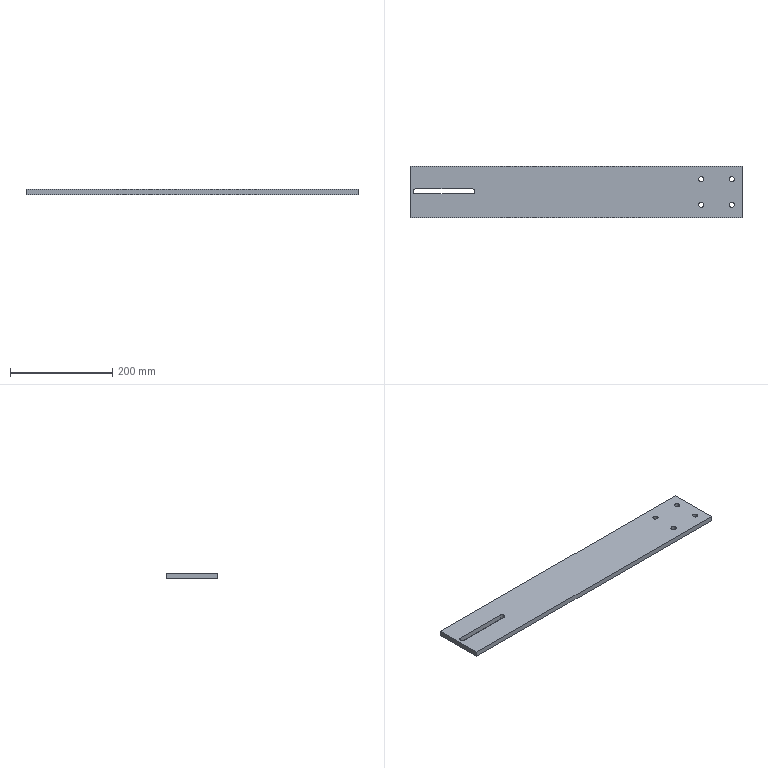Part | SolidWorks | features ICE 2, Extrusion 1 | 1 solid | 22 faces | box 650 x 100 x 10 mm | volume 635032 mm3 | cylinder 12 | plane 10 | commonest cylinder face diameters 10 x8 9 x4
STEP:
#1=CARTESIAN_POINT('',(300.,-25.,0.));
#2=VERTEX_POINT('',#1);
#3=CARTESIAN_POINT('',(310.,-25.,0.));
#4=VERTEX_POINT('',#3);
#5=CARTESIAN_POINT('',(305.,-25.,0.));
#6=DIRECTION('',(0.,0.,1.));
#7=DIRECTION('',(1.,0.,0.));
#8=AXIS2_PLACEMENT_3D('',#5,#6,#7);
#9=CIRCLE('',#8,5.);
#10=EDGE_CURVE('',#2,#4,#9,.T.);
#11=ORIENTED_EDGE('',*,*,#10,.F.);
#12=CARTESIAN_POINT('',(300.,-25.,10.));
#13=VERTEX_POINT('',#12);
#14=CARTESIAN_POINT('',(300.,-25.,0.));
#15=DIRECTION('',(0.,0.,1.));
#16=VECTOR('',#15,1000.);
#17=LINE('',#14,#16);
#18=EDGE_CURVE('',#2,#13,#17,.T.);
#19=ORIENTED_EDGE('',*,*,#18,.T.);
#20=CARTESIAN_POINT('',(310.,-25.,10.));
#21=VERTEX_POINT('',#20);
#22=CARTESIAN_POINT('',(305.,-25.,10.));
#23=DIRECTION('',(0.,0.,1.));
#24=DIRECTION('',(1.,0.,0.));
#25=AXIS2_PLACEMENT_3D('',#22,#23,#24);
#26=CIRCLE('',#25,5.);
#27=EDGE_CURVE('',#13,#21,#26,.T.);
#28=ORIENTED_EDGE('',*,*,#27,.T.);
#29=CARTESIAN_POINT('',(310.,-25.,0.));
#30=DIRECTION('',(0.,0.,1.));
#31=VECTOR('',#30,1000.);
#32=LINE('',#29,#31);
#33=EDGE_CURVE('',#4,#21,#32,.T.);
#34=ORIENTED_EDGE('',*,*,#33,.F.);
#35=EDGE_LOOP('',(#11,#19,#28,#34));
#36=FACE_OUTER_BOUND('',#35,.T.);
#37=CARTESIAN_POINT('',(305.,-25.,0.));
#38=DIRECTION('',(0.,0.,1.));
#39=DIRECTION('',(1.,0.,0.));
#40=AXIS2_PLACEMENT_3D('',#37,#38,#39);
#41=CYLINDRICAL_SURFACE('',#40,5.);
#42=ADVANCED_FACE('',(#36),#41,.F.);
#43=CARTESIAN_POINT('',(240.,-25.,0.));
#44=VERTEX_POINT('',#43);
#45=CARTESIAN_POINT('',(250.,-25.,0.));
#46=VERTEX_POINT('',#45);
#47=CARTESIAN_POINT('',(245.,-25.,0.));
#48=DIRECTION('',(0.,0.,1.));
#49=DIRECTION('',(1.,0.,0.));
#50=AXIS2_PLACEMENT_3D('',#47,#48,#49);
#51=CIRCLE('',#50,5.);
#52=EDGE_CURVE('',#44,#46,#51,.T.);
#53=ORIENTED_EDGE('',*,*,#52,.F.);
#54=CARTESIAN_POINT('',(240.,-25.,10.));
#55=VERTEX_POINT('',#54);
#56=CARTESIAN_POINT('',(240.,-25.,0.));
#57=DIRECTION('',(0.,0.,1.));
#58=VECTOR('',#57,1000.);
#59=LINE('',#56,#58);
#60=EDGE_CURVE('',#44,#55,#59,.T.);
#61=ORIENTED_EDGE('',*,*,#60,.T.);
#62=CARTESIAN_POINT('',(250.,-25.,10.));
#63=VERTEX_POINT('',#62);
#64=CARTESIAN_POINT('',(245.,-25.,10.));
#65=DIRECTION('',(0.,0.,1.));
#66=DIRECTION('',(1.,0.,0.));
#67=AXIS2_PLACEMENT_3D('',#64,#65,#66);
#68=CIRCLE('',#67,5.);
#69=EDGE_CURVE('',#55,#63,#68,.T.);
#70=ORIENTED_EDGE('',*,*,#69,.T.);
#71=CARTESIAN_POINT('',(250.,-25.,0.));
#72=DIRECTION('',(0.,0.,1.));
#73=VECTOR('',#72,1000.);
#74=LINE('',#71,#73);
#75=EDGE_CURVE('',#46,#63,#74,.T.);
#76=ORIENTED_EDGE('',*,*,#75,.F.);
#77=EDGE_LOOP('',(#53,#61,#70,#76));
#78=FACE_OUTER_BOUND('',#77,.T.);
#79=CARTESIAN_POINT('',(245.,-25.,0.));
#80=DIRECTION('',(0.,0.,1.));
#81=DIRECTION('',(1.,0.,0.));
#82=AXIS2_PLACEMENT_3D('',#79,#80,#81);
#83=CYLINDRICAL_SURFACE('',#82,5.);
#84=ADVANCED_FACE('',(#78),#83,.F.);
#85=CARTESIAN_POINT('',(240.,25.,0.));
#86=VERTEX_POINT('',#85);
#87=CARTESIAN_POINT('',(250.,25.,0.));
#88=VERTEX_POINT('',#87);
#89=CARTESIAN_POINT('',(245.,25.,0.));
#90=DIRECTION('',(0.,0.,1.));
#91=DIRECTION('',(1.,0.,0.));
#92=AXIS2_PLACEMENT_3D('',#89,#90,#91);
#93=CIRCLE('',#92,5.);
#94=EDGE_CURVE('',#86,#88,#93,.T.);
#95=ORIENTED_EDGE('',*,*,#94,.F.);
#96=CARTESIAN_POINT('',(240.,25.,10.));
#97=VERTEX_POINT('',#96);
#98=CARTESIAN_POINT('',(240.,25.,0.));
#99=DIRECTION('',(0.,0.,1.));
#100=VECTOR('',#99,1000.);
#101=LINE('',#98,#100);
#102=EDGE_CURVE('',#86,#97,#101,.T.);
#103=ORIENTED_EDGE('',*,*,#102,.T.);
#104=CARTESIAN_POINT('',(250.,25.,10.));
#105=VERTEX_POINT('',#104);
#106=CARTESIAN_POINT('',(245.,25.,10.));
#107=DIRECTION('',(0.,0.,1.));
#108=DIRECTION('',(1.,0.,0.));
#109=AXIS2_PLACEMENT_3D('',#106,#107,#108);
#110=CIRCLE('',#109,5.);
#111=EDGE_CURVE('',#97,#105,#110,.T.);
#112=ORIENTED_EDGE('',*,*,#111,.T.);
#113=CARTESIAN_POINT('',(250.,25.,0.));
#114=DIRECTION('',(0.,0.,1.));
#115=VECTOR('',#114,1000.);
#116=LINE('',#113,#115);
#117=EDGE_CURVE('',#88,#105,#116,.T.);
#118=ORIENTED_EDGE('',*,*,#117,.F.);
#119=EDGE_LOOP('',(#95,#103,#112,#118));
#120=FACE_OUTER_BOUND('',#119,.T.);
#121=CARTESIAN_POINT('',(245.,25.,0.));
#122=DIRECTION('',(0.,0.,1.));
#123=DIRECTION('',(1.,0.,0.));
#124=AXIS2_PLACEMENT_3D('',#121,#122,#123);
#125=CYLINDRICAL_SURFACE('',#124,5.);
#126=ADVANCED_FACE('',(#120),#125,.F.);
#127=CARTESIAN_POINT('',(300.,25.,0.));
#128=VERTEX_POINT('',#127);
#129=CARTESIAN_POINT('',(310.,25.,0.));
#130=VERTEX_POINT('',#129);
#131=CARTESIAN_POINT('',(305.,25.,0.));
#132=DIRECTION('',(0.,0.,1.));
#133=DIRECTION('',(1.,0.,0.));
#134=AXIS2_PLACEMENT_3D('',#131,#132,#133);
#135=CIRCLE('',#134,5.);
#136=EDGE_CURVE('',#128,#130,#135,.T.);
#137=ORIENTED_EDGE('',*,*,#136,.F.);
#138=CARTESIAN_POINT('',(300.,25.,10.));
#139=VERTEX_POINT('',#138);
#140=CARTESIAN_POINT('',(300.,25.,0.));
#141=DIRECTION('',(0.,0.,1.));
#142=VECTOR('',#141,1000.);
#143=LINE('',#140,#142);
#144=EDGE_CURVE('',#128,#139,#143,.T.);
#145=ORIENTED_EDGE('',*,*,#144,.T.);
#146=CARTESIAN_POINT('',(310.,25.,10.));
#147=VERTEX_POINT('',#146);
#148=CARTESIAN_POINT('',(305.,25.,10.));
#149=DIRECTION('',(0.,0.,1.));
#150=DIRECTION('',(1.,0.,0.));
#151=AXIS2_PLACEMENT_3D('',#148,#149,#150);
#152=CIRCLE('',#151,5.);
#153=EDGE_CURVE('',#139,#147,#152,.T.);
#154=ORIENTED_EDGE('',*,*,#153,.T.);
#155=CARTESIAN_POINT('',(310.,25.,0.));
#156=DIRECTION('',(0.,0.,1.));
#157=VECTOR('',#156,1000.);
#158=LINE('',#155,#157);
#159=EDGE_CURVE('',#130,#147,#158,.T.);
#160=ORIENTED_EDGE('',*,*,#159,.F.);
#161=EDGE_LOOP('',(#137,#145,#154,#160));
#162=FACE_OUTER_BOUND('',#161,.T.);
#163=CARTESIAN_POINT('',(305.,25.,0.));
#164=DIRECTION('',(0.,0.,1.));
#165=DIRECTION('',(1.,0.,0.));
#166=AXIS2_PLACEMENT_3D('',#163,#164,#165);
#167=CYLINDRICAL_SURFACE('',#166,5.);
#168=ADVANCED_FACE('',(#162),#167,.F.);
#169=CARTESIAN_POINT('',(-325.,50.,0.));
#170=VERTEX_POINT('',#169);
#171=CARTESIAN_POINT('',(-325.,-50.,0.));
#172=VERTEX_POINT('',#171);
#173=CARTESIAN_POINT('',(-325.,-50.,0.));
#174=DIRECTION('',(0.,-1.,0.));
#175=VECTOR('',#174,1000.);
#176=LINE('',#173,#175);
#177=EDGE_CURVE('',#170,#172,#176,.T.);
#178=ORIENTED_EDGE('',*,*,#177,.T.);
#179=CARTESIAN_POINT('',(-325.,-50.,10.));
#180=VERTEX_POINT('',#179);
#181=CARTESIAN_POINT('',(-325.,-50.,10.));
#182=DIRECTION('',(0.,0.,-1.));
#183=VECTOR('',#182,1000.);
#184=LINE('',#181,#183);
#185=EDGE_CURVE('',#180,#172,#184,.T.);
#186=ORIENTED_EDGE('',*,*,#185,.F.);
#187=CARTESIAN_POINT('',(-325.,50.,10.));
#188=VERTEX_POINT('',#187);
#189=CARTESIAN_POINT('',(-325.,-50.,10.));
#190=DIRECTION('',(0.,-1.,0.));
#191=VECTOR('',#190,1000.);
#192=LINE('',#189,#191);
#193=EDGE_CURVE('',#188,#180,#192,.T.);
#194=ORIENTED_EDGE('',*,*,#193,.F.);
#195=CARTESIAN_POINT('',(-325.,50.,10.));
#196=DIRECTION('',(0.,0.,-1.));
#197=VECTOR('',#196,1000.);
#198=LINE('',#195,#197);
#199=EDGE_CURVE('',#188,#170,#198,.T.);
#200=ORIENTED_EDGE('',*,*,#199,.T.);
#201=EDGE_LOOP('',(#178,#186,#194,#200));
#202=FACE_OUTER_BOUND('',#201,.T.);
#203=CARTESIAN_POINT('',(-325.,-50.,10.));
#204=DIRECTION('',(1.,0.,0.));
#205=DIRECTION('',(0.,0.,-1.));
#206=AXIS2_PLACEMENT_3D('',#203,#204,#205);
#207=PLANE('',#206);
#208=ADVANCED_FACE('',(#202),#207,.F.);
#209=CARTESIAN_POINT('',(325.,-50.,0.));
#210=VERTEX_POINT('',#209);
#211=CARTESIAN_POINT('',(325.,-50.,0.));
#212=DIRECTION('',(1.,0.,0.));
#213=VECTOR('',#212,1000.);
#214=LINE('',#211,#213);
#215=EDGE_CURVE('',#172,#210,#214,.T.);
#216=ORIENTED_EDGE('',*,*,#215,.T.);
#217=CARTESIAN_POINT('',(325.,-50.,10.));
#218=VERTEX_POINT('',#217);
#219=CARTESIAN_POINT('',(325.,-50.,10.));
#220=DIRECTION('',(0.,0.,-1.));
#221=VECTOR('',#220,1000.);
#222=LINE('',#219,#221);
#223=EDGE_CURVE('',#218,#210,#222,.T.);
#224=ORIENTED_EDGE('',*,*,#223,.F.);
#225=CARTESIAN_POINT('',(325.,-50.,10.));
#226=DIRECTION('',(1.,0.,0.));
#227=VECTOR('',#226,1000.);
#228=LINE('',#225,#227);
#229=EDGE_CURVE('',#180,#218,#228,.T.);
#230=ORIENTED_EDGE('',*,*,#229,.F.);
#231=ORIENTED_EDGE('',*,*,#185,.T.);
#232=EDGE_LOOP('',(#216,#224,#230,#231));
#233=FACE_OUTER_BOUND('',#232,.T.);
#234=CARTESIAN_POINT('',(325.,-50.,10.));
#235=DIRECTION('',(0.,1.,0.));
#236=DIRECTION('',(-1.,0.,0.));
#237=AXIS2_PLACEMENT_3D('',#234,#235,#236);
#238=PLANE('',#237);
#239=ADVANCED_FACE('',(#233),#238,.F.);
#240=CARTESIAN_POINT('',(325.,50.,0.));
#241=VERTEX_POINT('',#240);
#242=CARTESIAN_POINT('',(325.,-50.,0.));
#243=DIRECTION('',(0.,1.,0.));
#244=VECTOR('',#243,1000.);
#245=LINE('',#242,#244);
#246=EDGE_CURVE('',#210,#241,#245,.T.);
#247=ORIENTED_EDGE('',*,*,#246,.T.);
#248=CARTESIAN_POINT('',(325.,50.,10.));
#249=VERTEX_POINT('',#248);
#250=CARTESIAN_POINT('',(325.,50.,10.));
#251=DIRECTION('',(0.,0.,-1.));
#252=VECTOR('',#251,1000.);
#253=LINE('',#250,#252);
#254=EDGE_CURVE('',#249,#241,#253,.T.);
#255=ORIENTED_EDGE('',*,*,#254,.F.);
#256=CARTESIAN_POINT('',(325.,-50.,10.));
#257=DIRECTION('',(0.,1.,0.));
#258=VECTOR('',#257,1000.);
#259=LINE('',#256,#258);
#260=EDGE_CURVE('',#218,#249,#259,.T.);
#261=ORIENTED_EDGE('',*,*,#260,.F.);
#262=ORIENTED_EDGE('',*,*,#223,.T.);
#263=EDGE_LOOP('',(#247,#255,#261,#262));
#264=FACE_OUTER_BOUND('',#263,.T.);
#265=CARTESIAN_POINT('',(325.,-50.,10.));
#266=DIRECTION('',(-1.,0.,0.));
#267=DIRECTION('',(0.,0.,1.));
#268=AXIS2_PLACEMENT_3D('',#265,#266,#267);
#269=PLANE('',#268);
#270=ADVANCED_FACE('',(#264),#269,.F.);
#271=CARTESIAN_POINT('',(325.,50.,0.));
#272=DIRECTION('',(-1.,0.,0.));
#273=VECTOR('',#272,1000.);
#274=LINE('',#271,#273);
#275=EDGE_CURVE('',#241,#170,#274,.T.);
#276=ORIENTED_EDGE('',*,*,#275,.T.);
#277=ORIENTED_EDGE('',*,*,#199,.F.);
#278=CARTESIAN_POINT('',(325.,50.,10.));
#279=DIRECTION('',(-1.,0.,0.));
#280=VECTOR('',#279,1000.);
#281=LINE('',#278,#280);
#282=EDGE_CURVE('',#249,#188,#281,.T.);
#283=ORIENTED_EDGE('',*,*,#282,.F.);
#284=ORIENTED_EDGE('',*,*,#254,.T.);
#285=EDGE_LOOP('',(#276,#277,#283,#284));
#286=FACE_OUTER_BOUND('',#285,.T.);
#287=CARTESIAN_POINT('',(325.,50.,10.));
#288=DIRECTION('',(0.,-1.,0.));
#289=DIRECTION('',(1.,0.,0.));
#290=AXIS2_PLACEMENT_3D('',#287,#288,#289);
#291=PLANE('',#290);
#292=ADVANCED_FACE('',(#286),#291,.F.);
#293=CARTESIAN_POINT('',(-202.885,-3.814,10.));
#294=VERTEX_POINT('',#293);
#295=CARTESIAN_POINT('',(-198.385,0.6857,10.));
#296=VERTEX_POINT('',#295);
#297=CARTESIAN_POINT('',(-202.885,0.6857,10.));
#298=DIRECTION('',(0.,0.,1.));
#299=DIRECTION('',(1.,0.,0.));
#300=AXIS2_PLACEMENT_3D('',#297,#298,#299);
#301=CIRCLE('',#300,4.5);
#302=EDGE_CURVE('',#294,#296,#301,.T.);
#303=ORIENTED_EDGE('',*,*,#302,.F.);
#304=CARTESIAN_POINT('',(-313.885,-3.814,10.));
#305=VERTEX_POINT('',#304);
#306=CARTESIAN_POINT('',(-313.885,-3.814,10.));
#307=DIRECTION('',(1.,0.,0.));
#308=VECTOR('',#307,1000.);
#309=LINE('',#306,#308);
#310=EDGE_CURVE('',#305,#294,#309,.T.);
#311=ORIENTED_EDGE('',*,*,#310,.F.);
#312=CARTESIAN_POINT('',(-318.385,0.6857,10.));
#313=VERTEX_POINT('',#312);
#314=CARTESIAN_POINT('',(-313.885,0.6857,10.));
#315=DIRECTION('',(0.,0.,1.));
#316=DIRECTION('',(-1.,0.,0.));
#317=AXIS2_PLACEMENT_3D('',#314,#315,#316);
#318=CIRCLE('',#317,4.5);
#319=EDGE_CURVE('',#313,#305,#318,.T.);
#320=ORIENTED_EDGE('',*,*,#319,.F.);
#321=CARTESIAN_POINT('',(-318.385,1.686,10.));
#322=VERTEX_POINT('',#321);
#323=CARTESIAN_POINT('',(-318.385,0.6857,10.));
#324=DIRECTION('',(0.,-1.,0.));
#325=VECTOR('',#324,1000.);
#326=LINE('',#323,#325);
#327=EDGE_CURVE('',#322,#313,#326,.T.);
#328=ORIENTED_EDGE('',*,*,#327,.F.);
#329=CARTESIAN_POINT('',(-313.885,6.186,10.));
#330=VERTEX_POINT('',#329);
#331=CARTESIAN_POINT('',(-313.885,1.686,10.));
#332=DIRECTION('',(0.,0.,1.));
#333=DIRECTION('',(-1.,0.,0.));
#334=AXIS2_PLACEMENT_3D('',#331,#332,#333);
#335=CIRCLE('',#334,4.5);
#336=EDGE_CURVE('',#330,#322,#335,.T.);
#337=ORIENTED_EDGE('',*,*,#336,.F.);
#338=CARTESIAN_POINT('',(-202.885,6.186,10.));
#339=VERTEX_POINT('',#338);
#340=CARTESIAN_POINT('',(-313.885,6.186,10.));
#341=DIRECTION('',(-1.,0.,0.));
#342=VECTOR('',#341,1000.);
#343=LINE('',#340,#342);
#344=EDGE_CURVE('',#339,#330,#343,.T.);
#345=ORIENTED_EDGE('',*,*,#344,.F.);
#346=CARTESIAN_POINT('',(-198.385,1.686,10.));
#347=VERTEX_POINT('',#346);
#348=CARTESIAN_POINT('',(-202.885,1.686,10.));
#349=DIRECTION('',(0.,0.,1.));
#350=DIRECTION('',(-1.,0.,0.));
#351=AXIS2_PLACEMENT_3D('',#348,#349,#350);
#352=CIRCLE('',#351,4.5);
#353=EDGE_CURVE('',#347,#339,#352,.T.);
#354=ORIENTED_EDGE('',*,*,#353,.F.);
#355=CARTESIAN_POINT('',(-198.385,0.6857,10.));
#356=DIRECTION('',(0.,1.,0.));
#357=VECTOR('',#356,1000.);
#358=LINE('',#355,#357);
#359=EDGE_CURVE('',#296,#347,#358,.T.);
#360=ORIENTED_EDGE('',*,*,#359,.F.);
#361=EDGE_LOOP('',(#303,#311,#320,#328,#337,#345,#354,#360));
#362=FACE_BOUND('',#361,.T.);
#363=CARTESIAN_POINT('',(305.,-25.,10.));
#364=DIRECTION('',(0.,0.,1.));
#365=DIRECTION('',(1.,0.,0.));
#366=AXIS2_PLACEMENT_3D('',#363,#364,#365);
#367=CIRCLE('',#366,5.);
#368=EDGE_CURVE('',#21,#13,#367,.T.);
#369=ORIENTED_EDGE('',*,*,#368,.F.);
#370=ORIENTED_EDGE('',*,*,#27,.F.);
#371=EDGE_LOOP('',(#369,#370));
#372=FACE_BOUND('',#371,.T.);
#373=CARTESIAN_POINT('',(245.,-25.,10.));
#374=DIRECTION('',(0.,0.,1.));
#375=DIRECTION('',(1.,0.,0.));
#376=AXIS2_PLACEMENT_3D('',#373,#374,#375);
#377=CIRCLE('',#376,5.);
#378=EDGE_CURVE('',#63,#55,#377,.T.);
#379=ORIENTED_EDGE('',*,*,#378,.F.);
#380=ORIENTED_EDGE('',*,*,#69,.F.);
#381=EDGE_LOOP('',(#379,#380));
#382=FACE_BOUND('',#381,.T.);
#383=CARTESIAN_POINT('',(245.,25.,10.));
#384=DIRECTION('',(0.,0.,1.));
#385=DIRECTION('',(1.,0.,0.));
#386=AXIS2_PLACEMENT_3D('',#383,#384,#385);
#387=CIRCLE('',#386,5.);
#388=EDGE_CURVE('',#105,#97,#387,.T.);
#389=ORIENTED_EDGE('',*,*,#388,.F.);
#390=ORIENTED_EDGE('',*,*,#111,.F.);
#391=EDGE_LOOP('',(#389,#390));
#392=FACE_BOUND('',#391,.T.);
#393=CARTESIAN_POINT('',(305.,25.,10.));
#394=DIRECTION('',(0.,0.,1.));
#395=DIRECTION('',(1.,0.,0.));
#396=AXIS2_PLACEMENT_3D('',#393,#394,#395);
#397=CIRCLE('',#396,5.);
#398=EDGE_CURVE('',#147,#139,#397,.T.);
#399=ORIENTED_EDGE('',*,*,#398,.F.);
#400=ORIENTED_EDGE('',*,*,#153,.F.);
#401=EDGE_LOOP('',(#399,#400));
#402=FACE_BOUND('',#401,.T.);
#403=ORIENTED_EDGE('',*,*,#193,.T.);
#404=ORIENTED_EDGE('',*,*,#229,.T.);
#405=ORIENTED_EDGE('',*,*,#260,.T.);
#406=ORIENTED_EDGE('',*,*,#282,.T.);
#407=EDGE_LOOP('',(#403,#404,#405,#406));
#408=FACE_OUTER_BOUND('',#407,.T.);
#409=CARTESIAN_POINT('',(-325.,50.,10.));
#410=DIRECTION('',(0.,0.,1.));
#411=DIRECTION('',(1.,0.,0.));
#412=AXIS2_PLACEMENT_3D('',#409,#410,#411);
#413=PLANE('',#412);
#414=ADVANCED_FACE('',(#362,#372,#382,#392,#402,#408),#413,.T.);
#415=CARTESIAN_POINT('',(-313.885,-3.814,0.));
#416=VERTEX_POINT('',#415);
#417=CARTESIAN_POINT('',(-202.885,-3.814,0.));
#418=VERTEX_POINT('',#417);
#419=CARTESIAN_POINT('',(-313.885,-3.814,0.));
#420=DIRECTION('',(1.,0.,0.));
#421=VECTOR('',#420,1000.);
#422=LINE('',#419,#421);
#423=EDGE_CURVE('',#416,#418,#422,.T.);
#424=ORIENTED_EDGE('',*,*,#423,.T.);
#425=CARTESIAN_POINT('',(-198.385,0.6857,0.));
#426=VERTEX_POINT('',#425);
#427=CARTESIAN_POINT('',(-202.885,0.6857,0.));
#428=DIRECTION('',(0.,0.,1.));
#429=DIRECTION('',(1.,0.,0.));
#430=AXIS2_PLACEMENT_3D('',#427,#428,#429);
#431=CIRCLE('',#430,4.5);
#432=EDGE_CURVE('',#418,#426,#431,.T.);
#433=ORIENTED_EDGE('',*,*,#432,.T.);
#434=CARTESIAN_POINT('',(-198.385,1.686,0.));
#435=VERTEX_POINT('',#434);
#436=CARTESIAN_POINT('',(-198.385,0.6857,0.));
#437=DIRECTION('',(0.,1.,0.));
#438=VECTOR('',#437,1000.);
#439=LINE('',#436,#438);
#440=EDGE_CURVE('',#426,#435,#439,.T.);
#441=ORIENTED_EDGE('',*,*,#440,.T.);
#442=CARTESIAN_POINT('',(-202.885,6.186,0.));
#443=VERTEX_POINT('',#442);
#444=CARTESIAN_POINT('',(-202.885,1.686,0.));
#445=DIRECTION('',(0.,0.,1.));
#446=DIRECTION('',(-1.,0.,0.));
#447=AXIS2_PLACEMENT_3D('',#444,#445,#446);
#448=CIRCLE('',#447,4.5);
#449=EDGE_CURVE('',#435,#443,#448,.T.);
#450=ORIENTED_EDGE('',*,*,#449,.T.);
#451=CARTESIAN_POINT('',(-313.885,6.186,0.));
#452=VERTEX_POINT('',#451);
#453=CARTESIAN_POINT('',(-313.885,6.186,0.));
#454=DIRECTION('',(-1.,0.,0.));
#455=VECTOR('',#454,1000.);
#456=LINE('',#453,#455);
#457=EDGE_CURVE('',#443,#452,#456,.T.);
#458=ORIENTED_EDGE('',*,*,#457,.T.);
#459=CARTESIAN_POINT('',(-318.385,1.686,0.));
#460=VERTEX_POINT('',#459);
#461=CARTESIAN_POINT('',(-313.885,1.686,0.));
#462=DIRECTION('',(0.,0.,1.));
#463=DIRECTION('',(-1.,0.,0.));
#464=AXIS2_PLACEMENT_3D('',#461,#462,#463);
#465=CIRCLE('',#464,4.5);
#466=EDGE_CURVE('',#452,#460,#465,.T.);
#467=ORIENTED_EDGE('',*,*,#466,.T.);
#468=CARTESIAN_POINT('',(-318.385,0.6857,0.));
#469=VERTEX_POINT('',#468);
#470=CARTESIAN_POINT('',(-318.385,0.6857,0.));
#471=DIRECTION('',(0.,-1.,0.));
#472=VECTOR('',#471,1000.);
#473=LINE('',#470,#472);
#474=EDGE_CURVE('',#460,#469,#473,.T.);
#475=ORIENTED_EDGE('',*,*,#474,.T.);
#476=CARTESIAN_POINT('',(-313.885,0.6857,0.));
#477=DIRECTION('',(0.,0.,1.));
#478=DIRECTION('',(-1.,0.,0.));
#479=AXIS2_PLACEMENT_3D('',#476,#477,#478);
#480=CIRCLE('',#479,4.5);
#481=EDGE_CURVE('',#469,#416,#480,.T.);
#482=ORIENTED_EDGE('',*,*,#481,.T.);
#483=EDGE_LOOP('',(#424,#433,#441,#450,#458,#467,#475,#482));
#484=FACE_BOUND('',#483,.T.);
#485=CARTESIAN_POINT('',(305.,-25.,0.));
#486=DIRECTION('',(0.,0.,1.));
#487=DIRECTION('',(1.,0.,0.));
#488=AXIS2_PLACEMENT_3D('',#485,#486,#487);
#489=CIRCLE('',#488,5.);
#490=EDGE_CURVE('',#4,#2,#489,.T.);
#491=ORIENTED_EDGE('',*,*,#490,.T.);
#492=ORIENTED_EDGE('',*,*,#10,.T.);
#493=EDGE_LOOP('',(#491,#492));
#494=FACE_BOUND('',#493,.T.);
#495=CARTESIAN_POINT('',(245.,-25.,0.));
#496=DIRECTION('',(0.,0.,1.));
#497=DIRECTION('',(1.,0.,0.));
#498=AXIS2_PLACEMENT_3D('',#495,#496,#497);
#499=CIRCLE('',#498,5.);
#500=EDGE_CURVE('',#46,#44,#499,.T.);
#501=ORIENTED_EDGE('',*,*,#500,.T.);
#502=ORIENTED_EDGE('',*,*,#52,.T.);
#503=EDGE_LOOP('',(#501,#502));
#504=FACE_BOUND('',#503,.T.);
#505=CARTESIAN_POINT('',(245.,25.,0.));
#506=DIRECTION('',(0.,0.,1.));
#507=DIRECTION('',(1.,0.,0.));
#508=AXIS2_PLACEMENT_3D('',#505,#506,#507);
#509=CIRCLE('',#508,5.);
#510=EDGE_CURVE('',#88,#86,#509,.T.);
#511=ORIENTED_EDGE('',*,*,#510,.T.);
#512=ORIENTED_EDGE('',*,*,#94,.T.);
#513=EDGE_LOOP('',(#511,#512));
#514=FACE_BOUND('',#513,.T.);
#515=CARTESIAN_POINT('',(305.,25.,0.));
#516=DIRECTION('',(0.,0.,1.));
#517=DIRECTION('',(1.,0.,0.));
#518=AXIS2_PLACEMENT_3D('',#515,#516,#517);
#519=CIRCLE('',#518,5.);
#520=EDGE_CURVE('',#130,#128,#519,.T.);
#521=ORIENTED_EDGE('',*,*,#520,.T.);
#522=ORIENTED_EDGE('',*,*,#136,.T.);
#523=EDGE_LOOP('',(#521,#522));
#524=FACE_BOUND('',#523,.T.);
#525=ORIENTED_EDGE('',*,*,#177,.F.);
#526=ORIENTED_EDGE('',*,*,#275,.F.);
#527=ORIENTED_EDGE('',*,*,#246,.F.);
#528=ORIENTED_EDGE('',*,*,#215,.F.);
#529=EDGE_LOOP('',(#525,#526,#527,#528));
#530=FACE_OUTER_BOUND('',#529,.T.);
#531=CARTESIAN_POINT('',(-325.,50.,0.));
#532=DIRECTION('',(0.,0.,1.));
#533=DIRECTION('',(1.,0.,0.));
#534=AXIS2_PLACEMENT_3D('',#531,#532,#533);
#535=PLANE('',#534);
#536=ADVANCED_FACE('',(#484,#494,#504,#514,#524,#530),#535,.F.);
#537=ORIENTED_EDGE('',*,*,#144,.F.);
#538=ORIENTED_EDGE('',*,*,#520,.F.);
#539=ORIENTED_EDGE('',*,*,#159,.T.);
#540=ORIENTED_EDGE('',*,*,#398,.T.);
#541=EDGE_LOOP('',(#537,#538,#539,#540));
#542=FACE_OUTER_BOUND('',#541,.T.);
#543=CARTESIAN_POINT('',(305.,25.,0.));
#544=DIRECTION('',(0.,0.,1.));
#545=DIRECTION('',(1.,0.,0.));
#546=AXIS2_PLACEMENT_3D('',#543,#544,#545);
#547=CYLINDRICAL_SURFACE('',#546,5.);
#548=ADVANCED_FACE('',(#542),#547,.F.);
#549=ORIENTED_EDGE('',*,*,#102,.F.);
#550=ORIENTED_EDGE('',*,*,#510,.F.);
#551=ORIENTED_EDGE('',*,*,#117,.T.);
#552=ORIENTED_EDGE('',*,*,#388,.T.);
#553=EDGE_LOOP('',(#549,#550,#551,#552));
#554=FACE_OUTER_BOUND('',#553,.T.);
#555=CARTESIAN_POINT('',(245.,25.,0.));
#556=DIRECTION('',(0.,0.,1.));
#557=DIRECTION('',(1.,0.,0.));
#558=AXIS2_PLACEMENT_3D('',#555,#556,#557);
#559=CYLINDRICAL_SURFACE('',#558,5.);
#560=ADVANCED_FACE('',(#554),#559,.F.);
#561=ORIENTED_EDGE('',*,*,#60,.F.);
#562=ORIENTED_EDGE('',*,*,#500,.F.);
#563=ORIENTED_EDGE('',*,*,#75,.T.);
#564=ORIENTED_EDGE('',*,*,#378,.T.);
#565=EDGE_LOOP('',(#561,#562,#563,#564));
#566=FACE_OUTER_BOUND('',#565,.T.);
#567=CARTESIAN_POINT('',(245.,-25.,0.));
#568=DIRECTION('',(0.,0.,1.));
#569=DIRECTION('',(1.,0.,0.));
#570=AXIS2_PLACEMENT_3D('',#567,#568,#569);
#571=CYLINDRICAL_SURFACE('',#570,5.);
#572=ADVANCED_FACE('',(#566),#571,.F.);
#573=ORIENTED_EDGE('',*,*,#18,.F.);
#574=ORIENTED_EDGE('',*,*,#490,.F.);
#575=ORIENTED_EDGE('',*,*,#33,.T.);
#576=ORIENTED_EDGE('',*,*,#368,.T.);
#577=EDGE_LOOP('',(#573,#574,#575,#576));
#578=FACE_OUTER_BOUND('',#577,.T.);
#579=CARTESIAN_POINT('',(305.,-25.,0.));
#580=DIRECTION('',(0.,0.,1.));
#581=DIRECTION('',(1.,0.,0.));
#582=AXIS2_PLACEMENT_3D('',#579,#580,#581);
#583=CYLINDRICAL_SURFACE('',#582,5.);
#584=ADVANCED_FACE('',(#578),#583,.F.);
#585=ORIENTED_EDGE('',*,*,#302,.T.);
#586=CARTESIAN_POINT('',(-198.385,0.6857,0.));
#587=DIRECTION('',(0.,0.,1.));
#588=VECTOR('',#587,1000.);
#589=LINE('',#586,#588);
#590=EDGE_CURVE('',#426,#296,#589,.T.);
#591=ORIENTED_EDGE('',*,*,#590,.F.);
#592=ORIENTED_EDGE('',*,*,#432,.F.);
#593=CARTESIAN_POINT('',(-202.885,-3.814,0.));
#594=DIRECTION('',(0.,0.,1.));
#595=VECTOR('',#594,1000.);
#596=LINE('',#593,#595);
#597=EDGE_CURVE('',#418,#294,#596,.T.);
#598=ORIENTED_EDGE('',*,*,#597,.T.);
#599=EDGE_LOOP('',(#585,#591,#592,#598));
#600=FACE_OUTER_BOUND('',#599,.T.);
#601=CARTESIAN_POINT('',(-202.885,0.6857,0.));
#602=DIRECTION('',(0.,0.,1.));
#603=DIRECTION('',(1.,0.,0.));
#604=AXIS2_PLACEMENT_3D('',#601,#602,#603);
#605=CYLINDRICAL_SURFACE('',#604,4.5);
#606=ADVANCED_FACE('',(#600),#605,.F.);
#607=ORIENTED_EDGE('',*,*,#310,.T.);
#608=ORIENTED_EDGE('',*,*,#597,.F.);
#609=ORIENTED_EDGE('',*,*,#423,.F.);
#610=CARTESIAN_POINT('',(-313.885,-3.814,0.));
#611=DIRECTION('',(0.,0.,1.));
#612=VECTOR('',#611,1000.);
#613=LINE('',#610,#612);
#614=EDGE_CURVE('',#416,#305,#613,.T.);
#615=ORIENTED_EDGE('',*,*,#614,.T.);
#616=EDGE_LOOP('',(#607,#608,#609,#615));
#617=FACE_OUTER_BOUND('',#616,.T.);
#618=CARTESIAN_POINT('',(-313.885,-3.814,0.));
#619=DIRECTION('',(0.,-1.,0.));
#620=DIRECTION('',(0.,0.,-1.));
#621=AXIS2_PLACEMENT_3D('',#618,#619,#620);
#622=PLANE('',#621);
#623=ADVANCED_FACE('',(#617),#622,.F.);
#624=ORIENTED_EDGE('',*,*,#319,.T.);
#625=ORIENTED_EDGE('',*,*,#614,.F.);
#626=ORIENTED_EDGE('',*,*,#481,.F.);
#627=CARTESIAN_POINT('',(-318.385,0.6857,0.));
#628=DIRECTION('',(0.,0.,1.));
#629=VECTOR('',#628,1000.);
#630=LINE('',#627,#629);
#631=EDGE_CURVE('',#469,#313,#630,.T.);
#632=ORIENTED_EDGE('',*,*,#631,.T.);
#633=EDGE_LOOP('',(#624,#625,#626,#632));
#634=FACE_OUTER_BOUND('',#633,.T.);
#635=CARTESIAN_POINT('',(-313.885,0.6857,0.));
#636=DIRECTION('',(0.,0.,1.));
#637=DIRECTION('',(1.,0.,0.));
#638=AXIS2_PLACEMENT_3D('',#635,#636,#637);
#639=CYLINDRICAL_SURFACE('',#638,4.5);
#640=ADVANCED_FACE('',(#634),#639,.F.);
#641=ORIENTED_EDGE('',*,*,#327,.T.);
#642=ORIENTED_EDGE('',*,*,#631,.F.);
#643=ORIENTED_EDGE('',*,*,#474,.F.);
#644=CARTESIAN_POINT('',(-318.385,1.686,0.));
#645=DIRECTION('',(0.,0.,1.));
#646=VECTOR('',#645,1000.);
#647=LINE('',#644,#646);
#648=EDGE_CURVE('',#460,#322,#647,.T.);
#649=ORIENTED_EDGE('',*,*,#648,.T.);
#650=EDGE_LOOP('',(#641,#642,#643,#649));
#651=FACE_OUTER_BOUND('',#650,.T.);
#652=CARTESIAN_POINT('',(-318.385,0.6857,0.));
#653=DIRECTION('',(-1.,0.,0.));
#654=DIRECTION('',(0.,0.,1.));
#655=AXIS2_PLACEMENT_3D('',#652,#653,#654);
#656=PLANE('',#655);
#657=ADVANCED_FACE('',(#651),#656,.F.);
#658=ORIENTED_EDGE('',*,*,#336,.T.);
#659=ORIENTED_EDGE('',*,*,#648,.F.);
#660=ORIENTED_EDGE('',*,*,#466,.F.);
#661=CARTESIAN_POINT('',(-313.885,6.186,0.));
#662=DIRECTION('',(0.,0.,1.));
#663=VECTOR('',#662,1000.);
#664=LINE('',#661,#663);
#665=EDGE_CURVE('',#452,#330,#664,.T.);
#666=ORIENTED_EDGE('',*,*,#665,.T.);
#667=EDGE_LOOP('',(#658,#659,#660,#666));
#668=FACE_OUTER_BOUND('',#667,.T.);
#669=CARTESIAN_POINT('',(-313.885,1.686,0.));
#670=DIRECTION('',(0.,0.,1.));
#671=DIRECTION('',(1.,0.,0.));
#672=AXIS2_PLACEMENT_3D('',#669,#670,#671);
#673=CYLINDRICAL_SURFACE('',#672,4.5);
#674=ADVANCED_FACE('',(#668),#673,.F.);
#675=ORIENTED_EDGE('',*,*,#344,.T.);
#676=ORIENTED_EDGE('',*,*,#665,.F.);
#677=ORIENTED_EDGE('',*,*,#457,.F.);
#678=CARTESIAN_POINT('',(-202.885,6.186,0.));
#679=DIRECTION('',(0.,0.,1.));
#680=VECTOR('',#679,1000.);
#681=LINE('',#678,#680);
#682=EDGE_CURVE('',#443,#339,#681,.T.);
#683=ORIENTED_EDGE('',*,*,#682,.T.);
#684=EDGE_LOOP('',(#675,#676,#677,#683));
#685=FACE_OUTER_BOUND('',#684,.T.);
#686=CARTESIAN_POINT('',(-313.885,6.186,0.));
#687=DIRECTION('',(0.,1.,0.));
#688=DIRECTION('',(0.,0.,1.));
#689=AXIS2_PLACEMENT_3D('',#686,#687,#688);
#690=PLANE('',#689);
#691=ADVANCED_FACE('',(#685),#690,.F.);
#692=ORIENTED_EDGE('',*,*,#353,.T.);
#693=ORIENTED_EDGE('',*,*,#682,.F.);
#694=ORIENTED_EDGE('',*,*,#449,.F.);
#695=CARTESIAN_POINT('',(-198.385,1.686,0.));
#696=DIRECTION('',(0.,0.,1.));
#697=VECTOR('',#696,1000.);
#698=LINE('',#695,#697);
#699=EDGE_CURVE('',#435,#347,#698,.T.);
#700=ORIENTED_EDGE('',*,*,#699,.T.);
#701=EDGE_LOOP('',(#692,#693,#694,#700));
#702=FACE_OUTER_BOUND('',#701,.T.);
#703=CARTESIAN_POINT('',(-202.885,1.686,0.));
#704=DIRECTION('',(0.,0.,1.));
#705=DIRECTION('',(1.,0.,0.));
#706=AXIS2_PLACEMENT_3D('',#703,#704,#705);
#707=CYLINDRICAL_SURFACE('',#706,4.5);
#708=ADVANCED_FACE('',(#702),#707,.F.);
#709=ORIENTED_EDGE('',*,*,#359,.T.);
#710=ORIENTED_EDGE('',*,*,#699,.F.);
#711=ORIENTED_EDGE('',*,*,#440,.F.);
#712=ORIENTED_EDGE('',*,*,#590,.T.);
#713=EDGE_LOOP('',(#709,#710,#711,#712));
#714=FACE_OUTER_BOUND('',#713,.T.);
#715=CARTESIAN_POINT('',(-198.385,0.6857,0.));
#716=DIRECTION('',(1.,0.,0.));
#717=DIRECTION('',(0.,0.,-1.));
#718=AXIS2_PLACEMENT_3D('',#715,#716,#717);
#719=PLANE('',#718);
#720=ADVANCED_FACE('',(#714),#719,.F.);
#721=CLOSED_SHELL('',(#42,#84,#126,#168,#208,#239,#270,#292,#414,#536,#548,#560,#572,#584,#606,#623,#640,#657,#674,#691,#708,#720));
#722=MANIFOLD_SOLID_BREP('',#721);
#723=CARTESIAN_POINT('',(0.,0.,0.));
#724=DIRECTION('',(0.,0.,1.));
#725=DIRECTION('',(1.,0.,0.));
#726=AXIS2_PLACEMENT_3D('',#723,#724,#725);
#727=(LENGTH_UNIT()NAMED_UNIT(*)SI_UNIT(.MILLI.,.METRE.));
#728=UNCERTAINTY_MEASURE_WITH_UNIT(LENGTH_MEASURE(0.00001),#727,'','');
#729=(NAMED_UNIT(*)PLANE_ANGLE_UNIT()SI_UNIT($,.RADIAN.));
#730=(NAMED_UNIT(*)SI_UNIT($,.STERADIAN.)SOLID_ANGLE_UNIT());
#731=(GEOMETRIC_REPRESENTATION_CONTEXT(3)GLOBAL_UNCERTAINTY_ASSIGNED_CONTEXT((#728))GLOBAL_UNIT_ASSIGNED_CONTEXT((#727,#729,#730))REPRESENTATION_CONTEXT('',''));
#732=ADVANCED_BREP_SHAPE_REPRESENTATION('',(#722,#726),#731);